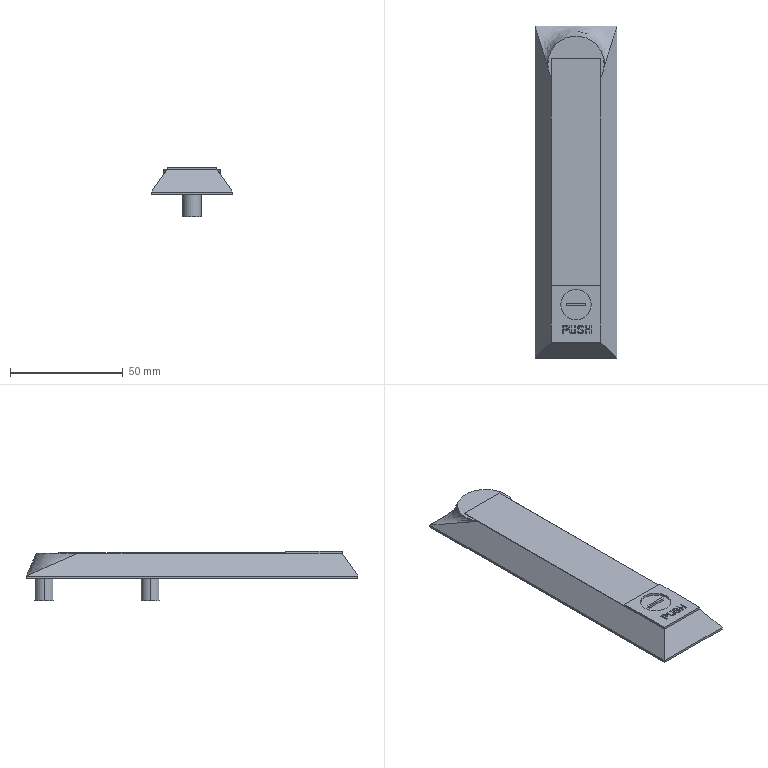Part | SolidWorks | features ICE 7, Blend 1 | 1 solid | 86 faces | box 36 x 147 x 22 mm | volume 47748 mm3 | plane 59 | spline 21 | cylinder 6 | commonest cylinder face diameters 8.179 x4 13.466 x2